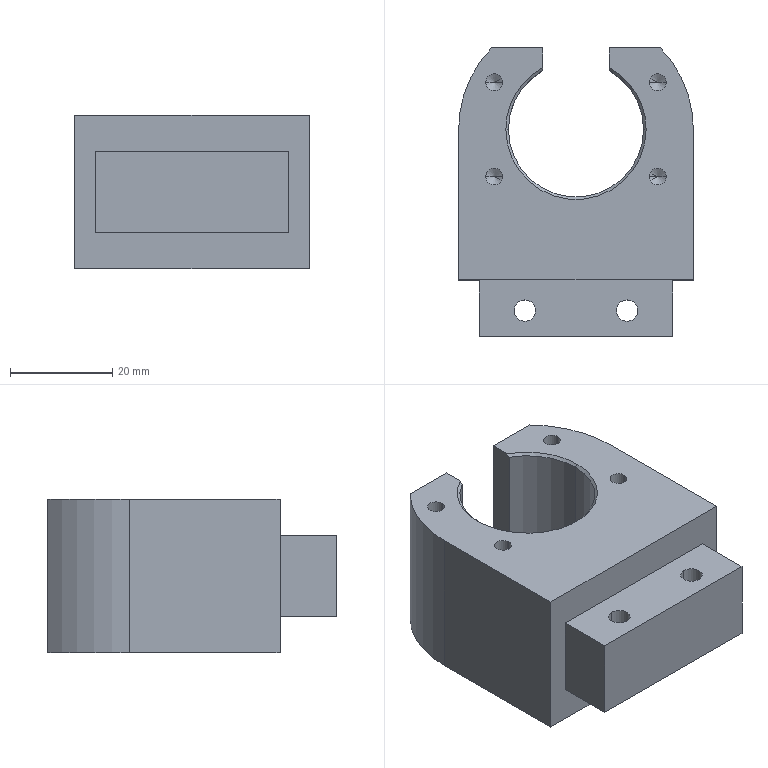Part | NX | features BREP 1 | 1 solid | 45 faces | box 46 x 56.5 x 30 mm | volume 48886 mm3 | cylinder 17 | plane 14 | cone 14 | commonest cylinder face diameters 3.3 x8 4.2 x4 26.5 x3 46 x2
STEP:
#1=CARTESIAN_POINT('',(10.,-37.6,7.));
#2=VERTEX_POINT('',#1);
#3=CARTESIAN_POINT('',(10.,-37.6,23.));
#4=VERTEX_POINT('',#3);
#5=CARTESIAN_POINT('',(10.,-37.6,7.));
#6=DIRECTION('',(0.,0.,-1.));
#7=VECTOR('',#6,1000.);
#8=LINE('',#5,#7);
#9=EDGE_CURVE('',#2,#4,#8,.F.);
#10=ORIENTED_EDGE('',*,*,#9,.T.);
#11=CARTESIAN_POINT('',(10.,-33.4,23.));
#12=VERTEX_POINT('',#11);
#13=CARTESIAN_POINT('',(10.,-35.5,23.));
#14=DIRECTION('',(0.,0.,1.));
#15=DIRECTION('',(1.,0.,0.));
#16=AXIS2_PLACEMENT_3D('',#13,#14,#15);
#17=CIRCLE('',#16,2.1);
#18=EDGE_CURVE('',#4,#12,#17,.T.);
#19=ORIENTED_EDGE('',*,*,#18,.T.);
#20=CARTESIAN_POINT('',(10.,-33.4,7.));
#21=VERTEX_POINT('',#20);
#22=CARTESIAN_POINT('',(10.,-33.4,7.));
#23=DIRECTION('',(0.,0.,-1.));
#24=VECTOR('',#23,1000.);
#25=LINE('',#22,#24);
#26=EDGE_CURVE('',#21,#12,#25,.F.);
#27=ORIENTED_EDGE('',*,*,#26,.F.);
#28=CARTESIAN_POINT('',(10.,-35.5,7.));
#29=DIRECTION('',(0.,0.,-1.));
#30=DIRECTION('',(0.,1.,0.));
#31=AXIS2_PLACEMENT_3D('',#28,#29,#30);
#32=CIRCLE('',#31,2.1);
#33=EDGE_CURVE('',#21,#2,#32,.T.);
#34=ORIENTED_EDGE('',*,*,#33,.T.);
#35=EDGE_LOOP('',(#10,#19,#27,#34));
#36=FACE_BOUND('',#35,.T.);
#37=CARTESIAN_POINT('',(10.,-35.5,7.));
#38=DIRECTION('',(0.,0.,-1.));
#39=DIRECTION('',(0.,1.,0.));
#40=AXIS2_PLACEMENT_3D('',#37,#38,#39);
#41=CYLINDRICAL_SURFACE('',#40,2.1);
#42=ADVANCED_FACE('',(#36),#41,.F.);
#43=CARTESIAN_POINT('',(-10.,-37.6,7.));
#44=VERTEX_POINT('',#43);
#45=CARTESIAN_POINT('',(-10.,-37.6,23.));
#46=VERTEX_POINT('',#45);
#47=CARTESIAN_POINT('',(-10.,-37.6,7.));
#48=DIRECTION('',(0.,0.,-1.));
#49=VECTOR('',#48,1000.);
#50=LINE('',#47,#49);
#51=EDGE_CURVE('',#44,#46,#50,.F.);
#52=ORIENTED_EDGE('',*,*,#51,.T.);
#53=CARTESIAN_POINT('',(-10.,-33.4,23.));
#54=VERTEX_POINT('',#53);
#55=CARTESIAN_POINT('',(-10.,-35.5,23.));
#56=DIRECTION('',(0.,0.,1.));
#57=DIRECTION('',(1.,0.,0.));
#58=AXIS2_PLACEMENT_3D('',#55,#56,#57);
#59=CIRCLE('',#58,2.1);
#60=EDGE_CURVE('',#46,#54,#59,.T.);
#61=ORIENTED_EDGE('',*,*,#60,.T.);
#62=CARTESIAN_POINT('',(-10.,-33.4,7.));
#63=VERTEX_POINT('',#62);
#64=CARTESIAN_POINT('',(-10.,-33.4,7.));
#65=DIRECTION('',(0.,0.,-1.));
#66=VECTOR('',#65,1000.);
#67=LINE('',#64,#66);
#68=EDGE_CURVE('',#63,#54,#67,.F.);
#69=ORIENTED_EDGE('',*,*,#68,.F.);
#70=CARTESIAN_POINT('',(-10.,-35.5,7.));
#71=DIRECTION('',(0.,0.,-1.));
#72=DIRECTION('',(0.,1.,0.));
#73=AXIS2_PLACEMENT_3D('',#70,#71,#72);
#74=CIRCLE('',#73,2.1);
#75=EDGE_CURVE('',#63,#44,#74,.T.);
#76=ORIENTED_EDGE('',*,*,#75,.T.);
#77=EDGE_LOOP('',(#52,#61,#69,#76));
#78=FACE_BOUND('',#77,.T.);
#79=CARTESIAN_POINT('',(-10.,-35.5,7.));
#80=DIRECTION('',(0.,0.,-1.));
#81=DIRECTION('',(0.,1.,0.));
#82=AXIS2_PLACEMENT_3D('',#79,#80,#81);
#83=CYLINDRICAL_SURFACE('',#82,2.1);
#84=ADVANCED_FACE('',(#78),#83,.F.);
#85=CARTESIAN_POINT('',(19.,-40.5,23.));
#86=VERTEX_POINT('',#85);
#87=CARTESIAN_POINT('',(-19.,-40.5,23.));
#88=VERTEX_POINT('',#87);
#89=CARTESIAN_POINT('',(19.,-40.5,23.));
#90=DIRECTION('',(-1.,0.,0.));
#91=VECTOR('',#90,1000.);
#92=LINE('',#89,#91);
#93=EDGE_CURVE('',#86,#88,#92,.T.);
#94=ORIENTED_EDGE('',*,*,#93,.T.);
#95=CARTESIAN_POINT('',(-19.,-40.5,7.));
#96=VERTEX_POINT('',#95);
#97=CARTESIAN_POINT('',(-19.,-40.5,23.));
#98=DIRECTION('',(0.,0.,-1.));
#99=VECTOR('',#98,1000.);
#100=LINE('',#97,#99);
#101=EDGE_CURVE('',#88,#96,#100,.T.);
#102=ORIENTED_EDGE('',*,*,#101,.T.);
#103=CARTESIAN_POINT('',(19.,-40.5,7.));
#104=VERTEX_POINT('',#103);
#105=CARTESIAN_POINT('',(19.,-40.5,7.));
#106=DIRECTION('',(1.,0.,0.));
#107=VECTOR('',#106,1000.);
#108=LINE('',#105,#107);
#109=EDGE_CURVE('',#96,#104,#108,.T.);
#110=ORIENTED_EDGE('',*,*,#109,.T.);
#111=CARTESIAN_POINT('',(19.,-40.5,23.));
#112=DIRECTION('',(0.,0.,1.));
#113=VECTOR('',#112,1000.);
#114=LINE('',#111,#113);
#115=EDGE_CURVE('',#104,#86,#114,.T.);
#116=ORIENTED_EDGE('',*,*,#115,.T.);
#117=EDGE_LOOP('',(#94,#102,#110,#116));
#118=FACE_BOUND('',#117,.T.);
#119=CARTESIAN_POINT('',(23.,-40.5,-61.288));
#120=DIRECTION('',(0.,-1.,0.));
#121=DIRECTION('',(1.,0.,0.));
#122=AXIS2_PLACEMENT_3D('',#119,#120,#121);
#123=PLANE('',#122);
#124=ADVANCED_FACE('',(#118),#123,.T.);
#125=ORIENTED_EDGE('',*,*,#109,.F.);
#126=CARTESIAN_POINT('',(-19.,-29.5,7.));
#127=VERTEX_POINT('',#126);
#128=CARTESIAN_POINT('',(-19.,-29.5,7.));
#129=DIRECTION('',(0.,-1.,0.));
#130=VECTOR('',#129,1000.);
#131=LINE('',#128,#130);
#132=EDGE_CURVE('',#127,#96,#131,.T.);
#133=ORIENTED_EDGE('',*,*,#132,.F.);
#134=CARTESIAN_POINT('',(19.,-29.5,7.));
#135=VERTEX_POINT('',#134);
#136=CARTESIAN_POINT('',(19.,-29.5,7.));
#137=DIRECTION('',(1.,0.,0.));
#138=VECTOR('',#137,1000.);
#139=LINE('',#136,#138);
#140=EDGE_CURVE('',#127,#135,#139,.T.);
#141=ORIENTED_EDGE('',*,*,#140,.T.);
#142=CARTESIAN_POINT('',(19.,-29.5,7.));
#143=DIRECTION('',(0.,-1.,0.));
#144=VECTOR('',#143,1000.);
#145=LINE('',#142,#144);
#146=EDGE_CURVE('',#135,#104,#145,.T.);
#147=ORIENTED_EDGE('',*,*,#146,.T.);
#148=EDGE_LOOP('',(#125,#133,#141,#147));
#149=FACE_BOUND('',#148,.T.);
#150=ORIENTED_EDGE('',*,*,#75,.F.);
#151=CARTESIAN_POINT('',(-10.,-35.5,7.));
#152=DIRECTION('',(0.,0.,-1.));
#153=DIRECTION('',(0.,1.,0.));
#154=AXIS2_PLACEMENT_3D('',#151,#152,#153);
#155=CIRCLE('',#154,2.1);
#156=EDGE_CURVE('',#44,#63,#155,.T.);
#157=ORIENTED_EDGE('',*,*,#156,.F.);
#158=EDGE_LOOP('',(#150,#157));
#159=FACE_BOUND('',#158,.T.);
#160=ORIENTED_EDGE('',*,*,#33,.F.);
#161=CARTESIAN_POINT('',(10.,-35.5,7.));
#162=DIRECTION('',(0.,0.,-1.));
#163=DIRECTION('',(0.,1.,0.));
#164=AXIS2_PLACEMENT_3D('',#161,#162,#163);
#165=CIRCLE('',#164,2.1);
#166=EDGE_CURVE('',#2,#21,#165,.T.);
#167=ORIENTED_EDGE('',*,*,#166,.F.);
#168=EDGE_LOOP('',(#160,#167));
#169=FACE_BOUND('',#168,.T.);
#170=CARTESIAN_POINT('',(19.,-29.5,7.));
#171=DIRECTION('',(0.,0.,-1.));
#172=DIRECTION('',(-1.,0.,0.));
#173=AXIS2_PLACEMENT_3D('',#170,#171,#172);
#174=PLANE('',#173);
#175=ADVANCED_FACE('',(#149,#159,#169),#174,.T.);
#176=ORIENTED_EDGE('',*,*,#115,.F.);
#177=ORIENTED_EDGE('',*,*,#146,.F.);
#178=CARTESIAN_POINT('',(19.,-29.5,23.));
#179=VERTEX_POINT('',#178);
#180=CARTESIAN_POINT('',(19.,-29.5,23.));
#181=DIRECTION('',(0.,0.,1.));
#182=VECTOR('',#181,1000.);
#183=LINE('',#180,#182);
#184=EDGE_CURVE('',#135,#179,#183,.T.);
#185=ORIENTED_EDGE('',*,*,#184,.T.);
#186=CARTESIAN_POINT('',(19.,-29.5,23.));
#187=DIRECTION('',(0.,-1.,0.));
#188=VECTOR('',#187,1000.);
#189=LINE('',#186,#188);
#190=EDGE_CURVE('',#179,#86,#189,.T.);
#191=ORIENTED_EDGE('',*,*,#190,.T.);
#192=EDGE_LOOP('',(#176,#177,#185,#191));
#193=FACE_BOUND('',#192,.T.);
#194=CARTESIAN_POINT('',(19.,-29.5,23.));
#195=DIRECTION('',(1.,0.,0.));
#196=DIRECTION('',(0.,0.,-1.));
#197=AXIS2_PLACEMENT_3D('',#194,#195,#196);
#198=PLANE('',#197);
#199=ADVANCED_FACE('',(#193),#198,.T.);
#200=ORIENTED_EDGE('',*,*,#93,.F.);
#201=ORIENTED_EDGE('',*,*,#190,.F.);
#202=CARTESIAN_POINT('',(-19.,-29.5,23.));
#203=VERTEX_POINT('',#202);
#204=CARTESIAN_POINT('',(19.,-29.5,23.));
#205=DIRECTION('',(-1.,0.,0.));
#206=VECTOR('',#205,1000.);
#207=LINE('',#204,#206);
#208=EDGE_CURVE('',#179,#203,#207,.T.);
#209=ORIENTED_EDGE('',*,*,#208,.T.);
#210=CARTESIAN_POINT('',(-19.,-29.5,23.));
#211=DIRECTION('',(0.,-1.,0.));
#212=VECTOR('',#211,1000.);
#213=LINE('',#210,#212);
#214=EDGE_CURVE('',#203,#88,#213,.T.);
#215=ORIENTED_EDGE('',*,*,#214,.T.);
#216=EDGE_LOOP('',(#200,#201,#209,#215));
#217=FACE_BOUND('',#216,.T.);
#218=CARTESIAN_POINT('',(-10.,-35.5,23.));
#219=DIRECTION('',(0.,0.,1.));
#220=DIRECTION('',(1.,0.,0.));
#221=AXIS2_PLACEMENT_3D('',#218,#219,#220);
#222=CIRCLE('',#221,2.1);
#223=EDGE_CURVE('',#54,#46,#222,.T.);
#224=ORIENTED_EDGE('',*,*,#223,.F.);
#225=ORIENTED_EDGE('',*,*,#60,.F.);
#226=EDGE_LOOP('',(#224,#225));
#227=FACE_BOUND('',#226,.T.);
#228=CARTESIAN_POINT('',(10.,-35.5,23.));
#229=DIRECTION('',(0.,0.,1.));
#230=DIRECTION('',(1.,0.,0.));
#231=AXIS2_PLACEMENT_3D('',#228,#229,#230);
#232=CIRCLE('',#231,2.1);
#233=EDGE_CURVE('',#12,#4,#232,.T.);
#234=ORIENTED_EDGE('',*,*,#233,.F.);
#235=ORIENTED_EDGE('',*,*,#18,.F.);
#236=EDGE_LOOP('',(#234,#235));
#237=FACE_BOUND('',#236,.T.);
#238=CARTESIAN_POINT('',(19.,-29.5,23.));
#239=DIRECTION('',(0.,0.,1.));
#240=DIRECTION('',(1.,0.,0.));
#241=AXIS2_PLACEMENT_3D('',#238,#239,#240);
#242=PLANE('',#241);
#243=ADVANCED_FACE('',(#217,#227,#237),#242,.T.);
#244=ORIENTED_EDGE('',*,*,#101,.F.);
#245=ORIENTED_EDGE('',*,*,#214,.F.);
#246=CARTESIAN_POINT('',(-19.,-29.5,23.));
#247=DIRECTION('',(0.,0.,-1.));
#248=VECTOR('',#247,1000.);
#249=LINE('',#246,#248);
#250=EDGE_CURVE('',#203,#127,#249,.T.);
#251=ORIENTED_EDGE('',*,*,#250,.T.);
#252=ORIENTED_EDGE('',*,*,#132,.T.);
#253=EDGE_LOOP('',(#244,#245,#251,#252));
#254=FACE_BOUND('',#253,.T.);
#255=CARTESIAN_POINT('',(-19.,-29.5,23.));
#256=DIRECTION('',(-1.,0.,0.));
#257=DIRECTION('',(0.,0.,1.));
#258=AXIS2_PLACEMENT_3D('',#255,#256,#257);
#259=PLANE('',#258);
#260=ADVANCED_FACE('',(#254),#259,.T.);
#261=ORIENTED_EDGE('',*,*,#208,.F.);
#262=ORIENTED_EDGE('',*,*,#184,.F.);
#263=ORIENTED_EDGE('',*,*,#140,.F.);
#264=ORIENTED_EDGE('',*,*,#250,.F.);
#265=EDGE_LOOP('',(#261,#262,#263,#264));
#266=FACE_BOUND('',#265,.T.);
#267=CARTESIAN_POINT('',(-23.,-29.5,30.));
#268=VERTEX_POINT('',#267);
#269=CARTESIAN_POINT('',(23.,-29.5,30.));
#270=VERTEX_POINT('',#269);
#271=CARTESIAN_POINT('',(0.,-29.5,30.));
#272=DIRECTION('',(1.,0.,0.));
#273=VECTOR('',#272,1000.);
#274=LINE('',#271,#273);
#275=EDGE_CURVE('',#268,#270,#274,.T.);
#276=ORIENTED_EDGE('',*,*,#275,.F.);
#277=CARTESIAN_POINT('',(-23.,-29.5,0.));
#278=VERTEX_POINT('',#277);
#279=CARTESIAN_POINT('',(-23.,-29.5,-61.288));
#280=DIRECTION('',(0.,0.,1.));
#281=VECTOR('',#280,1000.);
#282=LINE('',#279,#281);
#283=EDGE_CURVE('',#278,#268,#282,.T.);
#284=ORIENTED_EDGE('',*,*,#283,.F.);
#285=CARTESIAN_POINT('',(23.,-29.5,0.));
#286=VERTEX_POINT('',#285);
#287=CARTESIAN_POINT('',(0.,-29.5,0.));
#288=DIRECTION('',(1.,0.,0.));
#289=VECTOR('',#288,1000.);
#290=LINE('',#287,#289);
#291=EDGE_CURVE('',#278,#286,#290,.T.);
#292=ORIENTED_EDGE('',*,*,#291,.T.);
#293=CARTESIAN_POINT('',(23.,-29.5,-61.288));
#294=DIRECTION('',(0.,0.,-1.));
#295=VECTOR('',#294,1000.);
#296=LINE('',#293,#295);
#297=EDGE_CURVE('',#270,#286,#296,.T.);
#298=ORIENTED_EDGE('',*,*,#297,.F.);
#299=EDGE_LOOP('',(#276,#284,#292,#298));
#300=FACE_BOUND('',#299,.T.);
#301=CARTESIAN_POINT('',(0.,-29.5,15.));
#302=DIRECTION('',(0.,-1.,0.));
#303=DIRECTION('',(1.,0.,0.));
#304=AXIS2_PLACEMENT_3D('',#301,#302,#303);
#305=PLANE('',#304);
#306=ADVANCED_FACE('',(#266,#300),#305,.T.);
#307=CARTESIAN_POINT('',(-17.671,-9.25,30.));
#308=VERTEX_POINT('',#307);
#309=CARTESIAN_POINT('',(-17.671,-9.25,19.9));
#310=VERTEX_POINT('',#309);
#311=CARTESIAN_POINT('',(-17.671,-9.25,30.));
#312=DIRECTION('',(0.,0.,1.));
#313=VECTOR('',#312,1000.);
#314=LINE('',#311,#313);
#315=EDGE_CURVE('',#308,#310,#314,.F.);
#316=ORIENTED_EDGE('',*,*,#315,.T.);
#317=CARTESIAN_POINT('',(-14.371,-9.25,19.9));
#318=VERTEX_POINT('',#317);
#319=CARTESIAN_POINT('',(-16.021,-9.25,19.9));
#320=DIRECTION('',(0.,0.,1.));
#321=DIRECTION('',(1.,0.,0.));
#322=AXIS2_PLACEMENT_3D('',#319,#320,#321);
#323=CIRCLE('',#322,1.65);
#324=EDGE_CURVE('',#318,#310,#323,.T.);
#325=ORIENTED_EDGE('',*,*,#324,.F.);
#326=CARTESIAN_POINT('',(-14.371,-9.25,30.));
#327=VERTEX_POINT('',#326);
#328=CARTESIAN_POINT('',(-14.371,-9.25,30.));
#329=DIRECTION('',(0.,0.,1.));
#330=VECTOR('',#329,1000.);
#331=LINE('',#328,#330);
#332=EDGE_CURVE('',#327,#318,#331,.F.);
#333=ORIENTED_EDGE('',*,*,#332,.F.);
#334=CARTESIAN_POINT('',(-16.021,-9.25,30.));
#335=DIRECTION('',(0.,0.,1.));
#336=DIRECTION('',(1.,0.,0.));
#337=AXIS2_PLACEMENT_3D('',#334,#335,#336);
#338=CIRCLE('',#337,1.65);
#339=EDGE_CURVE('',#327,#308,#338,.T.);
#340=ORIENTED_EDGE('',*,*,#339,.T.);
#341=EDGE_LOOP('',(#316,#325,#333,#340));
#342=FACE_BOUND('',#341,.T.);
#343=CARTESIAN_POINT('',(-16.021,-9.25,30.));
#344=DIRECTION('',(0.,0.,1.));
#345=DIRECTION('',(1.,0.,0.));
#346=AXIS2_PLACEMENT_3D('',#343,#344,#345);
#347=CYLINDRICAL_SURFACE('',#346,1.65);
#348=ADVANCED_FACE('',(#342),#347,.F.);
#349=CARTESIAN_POINT('',(-16.021,-9.25,18.909));
#350=VERTEX_POINT('',#349);
#351=CARTESIAN_POINT('',(-17.671,-9.25,19.9));
#352=DIRECTION('',(-0.8572,0.,0.515));
#353=VECTOR('',#352,1000.);
#354=LINE('',#351,#353);
#355=EDGE_CURVE('',#350,#310,#354,.T.);
#356=ORIENTED_EDGE('',*,*,#355,.F.);
#357=CARTESIAN_POINT('',(-14.371,-9.25,19.9));
#358=DIRECTION('',(0.8572,0.,0.515));
#359=VECTOR('',#358,1000.);
#360=LINE('',#357,#359);
#361=EDGE_CURVE('',#350,#318,#360,.T.);
#362=ORIENTED_EDGE('',*,*,#361,.T.);
#363=ORIENTED_EDGE('',*,*,#324,.T.);
#364=EDGE_LOOP('',(#356,#362,#363));
#365=FACE_BOUND('',#364,.T.);
#366=CARTESIAN_POINT('',(-16.021,-9.25,19.9));
#367=DIRECTION('',(0.,0.,1.));
#368=DIRECTION('',(1.,0.,0.));
#369=AXIS2_PLACEMENT_3D('',#366,#367,#368);
#370=CONICAL_SURFACE('',#369,1.65,1.03);
#371=ADVANCED_FACE('',(#365),#370,.F.);
#372=CARTESIAN_POINT('',(14.371,9.25,30.));
#373=VERTEX_POINT('',#372);
#374=CARTESIAN_POINT('',(14.371,9.25,19.9));
#375=VERTEX_POINT('',#374);
#376=CARTESIAN_POINT('',(14.371,9.25,30.));
#377=DIRECTION('',(0.,0.,1.));
#378=VECTOR('',#377,1000.);
#379=LINE('',#376,#378);
#380=EDGE_CURVE('',#373,#375,#379,.F.);
#381=ORIENTED_EDGE('',*,*,#380,.T.);
#382=CARTESIAN_POINT('',(17.671,9.25,19.9));
#383=VERTEX_POINT('',#382);
#384=CARTESIAN_POINT('',(16.021,9.25,19.9));
#385=DIRECTION('',(0.,0.,1.));
#386=DIRECTION('',(1.,0.,0.));
#387=AXIS2_PLACEMENT_3D('',#384,#385,#386);
#388=CIRCLE('',#387,1.65);
#389=EDGE_CURVE('',#383,#375,#388,.T.);
#390=ORIENTED_EDGE('',*,*,#389,.F.);
#391=CARTESIAN_POINT('',(17.671,9.25,30.));
#392=VERTEX_POINT('',#391);
#393=CARTESIAN_POINT('',(17.671,9.25,30.));
#394=DIRECTION('',(0.,0.,1.));
#395=VECTOR('',#394,1000.);
#396=LINE('',#393,#395);
#397=EDGE_CURVE('',#392,#383,#396,.F.);
#398=ORIENTED_EDGE('',*,*,#397,.F.);
#399=CARTESIAN_POINT('',(16.021,9.25,30.));
#400=DIRECTION('',(0.,0.,1.));
#401=DIRECTION('',(1.,0.,0.));
#402=AXIS2_PLACEMENT_3D('',#399,#400,#401);
#403=CIRCLE('',#402,1.65);
#404=EDGE_CURVE('',#392,#373,#403,.T.);
#405=ORIENTED_EDGE('',*,*,#404,.T.);
#406=EDGE_LOOP('',(#381,#390,#398,#405));
#407=FACE_BOUND('',#406,.T.);
#408=CARTESIAN_POINT('',(16.021,9.25,30.));
#409=DIRECTION('',(0.,0.,1.));
#410=DIRECTION('',(1.,0.,0.));
#411=AXIS2_PLACEMENT_3D('',#408,#409,#410);
#412=CYLINDRICAL_SURFACE('',#411,1.65);
#413=ADVANCED_FACE('',(#407),#412,.F.);
#414=CARTESIAN_POINT('',(16.021,9.25,18.909));
#415=VERTEX_POINT('',#414);
#416=CARTESIAN_POINT('',(14.371,9.25,19.9));
#417=DIRECTION('',(-0.8572,0.,0.515));
#418=VECTOR('',#417,1000.);
#419=LINE('',#416,#418);
#420=EDGE_CURVE('',#415,#375,#419,.T.);
#421=ORIENTED_EDGE('',*,*,#420,.F.);
#422=CARTESIAN_POINT('',(17.671,9.25,19.9));
#423=DIRECTION('',(0.8572,0.,0.515));
#424=VECTOR('',#423,1000.);
#425=LINE('',#422,#424);
#426=EDGE_CURVE('',#415,#383,#425,.T.);
#427=ORIENTED_EDGE('',*,*,#426,.T.);
#428=ORIENTED_EDGE('',*,*,#389,.T.);
#429=EDGE_LOOP('',(#421,#427,#428));
#430=FACE_BOUND('',#429,.T.);
#431=CARTESIAN_POINT('',(16.021,9.25,19.9));
#432=DIRECTION('',(0.,0.,1.));
#433=DIRECTION('',(1.,0.,0.));
#434=AXIS2_PLACEMENT_3D('',#431,#432,#433);
#435=CONICAL_SURFACE('',#434,1.65,1.03);
#436=ADVANCED_FACE('',(#430),#435,.F.);
#437=CARTESIAN_POINT('',(14.371,-9.25,30.));
#438=VERTEX_POINT('',#437);
#439=CARTESIAN_POINT('',(14.371,-9.25,19.9));
#440=VERTEX_POINT('',#439);
#441=CARTESIAN_POINT('',(14.371,-9.25,30.));
#442=DIRECTION('',(0.,0.,1.));
#443=VECTOR('',#442,1000.);
#444=LINE('',#441,#443);
#445=EDGE_CURVE('',#438,#440,#444,.F.);
#446=ORIENTED_EDGE('',*,*,#445,.T.);
#447=CARTESIAN_POINT('',(17.671,-9.25,19.9));
#448=VERTEX_POINT('',#447);
#449=CARTESIAN_POINT('',(16.021,-9.25,19.9));
#450=DIRECTION('',(0.,0.,1.));
#451=DIRECTION('',(1.,0.,0.));
#452=AXIS2_PLACEMENT_3D('',#449,#450,#451);
#453=CIRCLE('',#452,1.65);
#454=EDGE_CURVE('',#448,#440,#453,.T.);
#455=ORIENTED_EDGE('',*,*,#454,.F.);
#456=CARTESIAN_POINT('',(17.671,-9.25,30.));
#457=VERTEX_POINT('',#456);
#458=CARTESIAN_POINT('',(17.671,-9.25,30.));
#459=DIRECTION('',(0.,0.,1.));
#460=VECTOR('',#459,1000.);
#461=LINE('',#458,#460);
#462=EDGE_CURVE('',#457,#448,#461,.F.);
#463=ORIENTED_EDGE('',*,*,#462,.F.);
#464=CARTESIAN_POINT('',(16.021,-9.25,30.));
#465=DIRECTION('',(0.,0.,1.));
#466=DIRECTION('',(1.,0.,0.));
#467=AXIS2_PLACEMENT_3D('',#464,#465,#466);
#468=CIRCLE('',#467,1.65);
#469=EDGE_CURVE('',#457,#438,#468,.T.);
#470=ORIENTED_EDGE('',*,*,#469,.T.);
#471=EDGE_LOOP('',(#446,#455,#463,#470));
#472=FACE_BOUND('',#471,.T.);
#473=CARTESIAN_POINT('',(16.021,-9.25,30.));
#474=DIRECTION('',(0.,0.,1.));
#475=DIRECTION('',(1.,0.,0.));
#476=AXIS2_PLACEMENT_3D('',#473,#474,#475);
#477=CYLINDRICAL_SURFACE('',#476,1.65);
#478=ADVANCED_FACE('',(#472),#477,.F.);
#479=CARTESIAN_POINT('',(16.021,-9.25,18.909));
#480=VERTEX_POINT('',#479);
#481=CARTESIAN_POINT('',(14.371,-9.25,19.9));
#482=DIRECTION('',(-0.8572,0.,0.515));
#483=VECTOR('',#482,1000.);
#484=LINE('',#481,#483);
#485=EDGE_CURVE('',#480,#440,#484,.T.);
#486=ORIENTED_EDGE('',*,*,#485,.F.);
#487=CARTESIAN_POINT('',(17.671,-9.25,19.9));
#488=DIRECTION('',(0.8572,0.,0.515));
#489=VECTOR('',#488,1000.);
#490=LINE('',#487,#489);
#491=EDGE_CURVE('',#480,#448,#490,.T.);
#492=ORIENTED_EDGE('',*,*,#491,.T.);
#493=ORIENTED_EDGE('',*,*,#454,.T.);
#494=EDGE_LOOP('',(#486,#492,#493));
#495=FACE_BOUND('',#494,.T.);
#496=CARTESIAN_POINT('',(16.021,-9.25,19.9));
#497=DIRECTION('',(0.,0.,1.));
#498=DIRECTION('',(1.,0.,0.));
#499=AXIS2_PLACEMENT_3D('',#496,#497,#498);
#500=CONICAL_SURFACE('',#499,1.65,1.03);
#501=ADVANCED_FACE('',(#495),#500,.F.);
#502=CARTESIAN_POINT('',(-17.671,9.25,30.));
#503=VERTEX_POINT('',#502);
#504=CARTESIAN_POINT('',(-17.671,9.25,19.9));
#505=VERTEX_POINT('',#504);
#506=CARTESIAN_POINT('',(-17.671,9.25,30.));
#507=DIRECTION('',(0.,0.,1.));
#508=VECTOR('',#507,1000.);
#509=LINE('',#506,#508);
#510=EDGE_CURVE('',#503,#505,#509,.F.);
#511=ORIENTED_EDGE('',*,*,#510,.T.);
#512=CARTESIAN_POINT('',(-14.371,9.25,19.9));
#513=VERTEX_POINT('',#512);
#514=CARTESIAN_POINT('',(-16.021,9.25,19.9));
#515=DIRECTION('',(0.,0.,1.));
#516=DIRECTION('',(1.,0.,0.));
#517=AXIS2_PLACEMENT_3D('',#514,#515,#516);
#518=CIRCLE('',#517,1.65);
#519=EDGE_CURVE('',#513,#505,#518,.T.);
#520=ORIENTED_EDGE('',*,*,#519,.F.);
#521=CARTESIAN_POINT('',(-14.371,9.25,30.));
#522=VERTEX_POINT('',#521);
#523=CARTESIAN_POINT('',(-14.371,9.25,30.));
#524=DIRECTION('',(0.,0.,1.));
#525=VECTOR('',#524,1000.);
#526=LINE('',#523,#525);
#527=EDGE_CURVE('',#522,#513,#526,.F.);
#528=ORIENTED_EDGE('',*,*,#527,.F.);
#529=CARTESIAN_POINT('',(-16.021,9.25,30.));
#530=DIRECTION('',(0.,0.,1.));
#531=DIRECTION('',(1.,0.,0.));
#532=AXIS2_PLACEMENT_3D('',#529,#530,#531);
#533=CIRCLE('',#532,1.65);
#534=EDGE_CURVE('',#522,#503,#533,.T.);
#535=ORIENTED_EDGE('',*,*,#534,.T.);
#536=EDGE_LOOP('',(#511,#520,#528,#535));
#537=FACE_BOUND('',#536,.T.);
#538=CARTESIAN_POINT('',(-16.021,9.25,30.));
#539=DIRECTION('',(0.,0.,1.));
#540=DIRECTION('',(1.,0.,0.));
#541=AXIS2_PLACEMENT_3D('',#538,#539,#540);
#542=CYLINDRICAL_SURFACE('',#541,1.65);
#543=ADVANCED_FACE('',(#537),#542,.F.);
#544=CARTESIAN_POINT('',(-16.021,9.25,18.909));
#545=VERTEX_POINT('',#544);
#546=CARTESIAN_POINT('',(-17.671,9.25,19.9));
#547=DIRECTION('',(-0.8572,0.,0.515));
#548=VECTOR('',#547,1000.);
#549=LINE('',#546,#548);
#550=EDGE_CURVE('',#545,#505,#549,.T.);
#551=ORIENTED_EDGE('',*,*,#550,.F.);
#552=CARTESIAN_POINT('',(-14.371,9.25,19.9));
#553=DIRECTION('',(0.8572,0.,0.515));
#554=VECTOR('',#553,1000.);
#555=LINE('',#552,#554);
#556=EDGE_CURVE('',#545,#513,#555,.T.);
#557=ORIENTED_EDGE('',*,*,#556,.T.);
#558=ORIENTED_EDGE('',*,*,#519,.T.);
#559=EDGE_LOOP('',(#551,#557,#558));
#560=FACE_BOUND('',#559,.T.);
#561=CARTESIAN_POINT('',(-16.021,9.25,19.9));
#562=DIRECTION('',(0.,0.,1.));
#563=DIRECTION('',(1.,0.,0.));
#564=AXIS2_PLACEMENT_3D('',#561,#562,#563);
#565=CONICAL_SURFACE('',#564,1.65,1.03);
#566=ADVANCED_FACE('',(#560),#565,.F.);
#567=CARTESIAN_POINT('',(-13.25,0.,29.5));
#568=VERTEX_POINT('',#567);
#569=CARTESIAN_POINT('',(-13.75,0.,30.));
#570=VERTEX_POINT('',#569);
#571=CARTESIAN_POINT('',(-13.75,0.,30.));
#572=DIRECTION('',(-0.7071,0.,0.7071));
#573=VECTOR('',#572,1000.);
#574=LINE('',#571,#573);
#575=EDGE_CURVE('',#568,#570,#574,.T.);
#576=ORIENTED_EDGE('',*,*,#575,.F.);
#577=CARTESIAN_POINT('',(-6.5,11.546,29.5));
#578=VERTEX_POINT('',#577);
#579=CARTESIAN_POINT('',(0.,0.,29.5));
#580=DIRECTION('',(0.,0.,1.));
#581=DIRECTION('',(1.,0.,0.));
#582=AXIS2_PLACEMENT_3D('',#579,#580,#581);
#583=CIRCLE('',#582,13.25);
#584=EDGE_CURVE('',#578,#568,#583,.T.);
#585=ORIENTED_EDGE('',*,*,#584,.F.);
#586=CARTESIAN_POINT('',(-6.5,12.117,30.));
#587=VERTEX_POINT('',#586);
#588=CARTESIAN_POINT('',(-6.5,12.117,30.));
#589=CARTESIAN_POINT('',(-6.5,11.927,29.833));
#590=CARTESIAN_POINT('',(-6.5,11.737,29.666));
#591=CARTESIAN_POINT('',(-6.5,11.546,29.5));
#592=B_SPLINE_CURVE_WITH_KNOTS('',3,(#588,#589,#590,#591),.UNSPECIFIED.,.F.,.F.,(4,4),(0.,0.0007586),.UNSPECIFIED.);
#593=EDGE_CURVE('',#587,#578,#592,.T.);
#594=ORIENTED_EDGE('',*,*,#593,.F.);
#595=CARTESIAN_POINT('',(0.,0.,30.));
#596=DIRECTION('',(0.,0.,-1.));
#597=DIRECTION('',(1.,0.,0.));
#598=AXIS2_PLACEMENT_3D('',#595,#596,#597);
#599=CIRCLE('',#598,13.75);
#600=EDGE_CURVE('',#570,#587,#599,.T.);
#601=ORIENTED_EDGE('',*,*,#600,.F.);
#602=EDGE_LOOP('',(#576,#585,#594,#601));
#603=FACE_BOUND('',#602,.T.);
#604=CARTESIAN_POINT('',(0.,0.,30.));
#605=DIRECTION('',(0.,0.,1.));
#606=DIRECTION('',(1.,0.,0.));
#607=AXIS2_PLACEMENT_3D('',#604,#605,#606);
#608=CONICAL_SURFACE('',#607,13.75,0.7854);
#609=ADVANCED_FACE('',(#603),#608,.F.);
#610=CARTESIAN_POINT('',(13.25,0.,0.5));
#611=VERTEX_POINT('',#610);
#612=CARTESIAN_POINT('',(13.75,0.,0.));
#613=VERTEX_POINT('',#612);
#614=CARTESIAN_POINT('',(13.25,0.,0.5));
#615=DIRECTION('',(0.7071,0.,-0.7071));
#616=VECTOR('',#615,1000.);
#617=LINE('',#614,#616);
#618=EDGE_CURVE('',#611,#613,#617,.T.);
#619=ORIENTED_EDGE('',*,*,#618,.F.);
#620=CARTESIAN_POINT('',(6.5,11.546,0.5));
#621=VERTEX_POINT('',#620);
#622=CARTESIAN_POINT('',(0.,0.,0.5));
#623=DIRECTION('',(0.,0.,-1.));
#624=DIRECTION('',(1.,0.,0.));
#625=AXIS2_PLACEMENT_3D('',#622,#623,#624);
#626=CIRCLE('',#625,13.25);
#627=EDGE_CURVE('',#621,#611,#626,.T.);
#628=ORIENTED_EDGE('',*,*,#627,.F.);
#629=CARTESIAN_POINT('',(6.5,12.117,0.));
#630=VERTEX_POINT('',#629);
#631=CARTESIAN_POINT('',(6.5,12.117,0.));
#632=CARTESIAN_POINT('',(6.5,11.927,0.1672));
#633=CARTESIAN_POINT('',(6.5,11.737,0.3339));
#634=CARTESIAN_POINT('',(6.5,11.546,0.5));
#635=B_SPLINE_CURVE_WITH_KNOTS('',3,(#631,#632,#633,#634),.UNSPECIFIED.,.F.,.F.,(4,4),(0.,0.0007586),.UNSPECIFIED.);
#636=EDGE_CURVE('',#630,#621,#635,.T.);
#637=ORIENTED_EDGE('',*,*,#636,.F.);
#638=CARTESIAN_POINT('',(0.,0.,0.));
#639=DIRECTION('',(0.,0.,1.));
#640=DIRECTION('',(1.,0.,0.));
#641=AXIS2_PLACEMENT_3D('',#638,#639,#640);
#642=CIRCLE('',#641,13.75);
#643=EDGE_CURVE('',#613,#630,#642,.T.);
#644=ORIENTED_EDGE('',*,*,#643,.F.);
#645=EDGE_LOOP('',(#619,#628,#637,#644));
#646=FACE_BOUND('',#645,.T.);
#647=CARTESIAN_POINT('',(0.,0.,0.5));
#648=DIRECTION('',(0.,0.,-1.));
#649=DIRECTION('',(-1.,0.,0.));
#650=AXIS2_PLACEMENT_3D('',#647,#648,#649);
#651=CONICAL_SURFACE('',#650,13.25,0.7854);
#652=ADVANCED_FACE('',(#646),#651,.F.);
#653=CARTESIAN_POINT('',(-16.523,16.,0.));
#654=VERTEX_POINT('',#653);
#655=CARTESIAN_POINT('',(-6.5,16.,0.));
#656=VERTEX_POINT('',#655);
#657=CARTESIAN_POINT('',(-16.523,16.,0.));
#658=DIRECTION('',(1.,0.,0.));
#659=VECTOR('',#658,1000.);
#660=LINE('',#657,#659);
#661=EDGE_CURVE('',#654,#656,#660,.T.);
#662=ORIENTED_EDGE('',*,*,#661,.F.);
#663=CARTESIAN_POINT('',(-16.523,16.,30.));
#664=VERTEX_POINT('',#663);
#665=CARTESIAN_POINT('',(-16.523,16.,0.));
#666=DIRECTION('',(0.,0.,1.));
#667=VECTOR('',#666,1000.);
#668=LINE('',#665,#667);
#669=EDGE_CURVE('',#654,#664,#668,.T.);
#670=ORIENTED_EDGE('',*,*,#669,.T.);
#671=CARTESIAN_POINT('',(-6.5,16.,30.));
#672=VERTEX_POINT('',#671);
#673=CARTESIAN_POINT('',(-16.523,16.,30.));
#674=DIRECTION('',(1.,0.,0.));
#675=VECTOR('',#674,1000.);
#676=LINE('',#673,#675);
#677=EDGE_CURVE('',#664,#672,#676,.T.);
#678=ORIENTED_EDGE('',*,*,#677,.T.);
#679=CARTESIAN_POINT('',(-6.5,16.,30.));
#680=DIRECTION('',(0.,0.,1.));
#681=VECTOR('',#680,1000.);
#682=LINE('',#679,#681);
#683=EDGE_CURVE('',#656,#672,#682,.T.);
#684=ORIENTED_EDGE('',*,*,#683,.F.);
#685=EDGE_LOOP('',(#662,#670,#678,#684));
#686=FACE_BOUND('',#685,.T.);
#687=CARTESIAN_POINT('',(-16.523,16.,0.));
#688=DIRECTION('',(0.,-1.,0.));
#689=DIRECTION('',(0.,0.,-1.));
#690=AXIS2_PLACEMENT_3D('',#687,#688,#689);
#691=PLANE('',#690);
#692=ADVANCED_FACE('',(#686),#691,.F.);
#693=CARTESIAN_POINT('',(6.5,16.,30.));
#694=VERTEX_POINT('',#693);
#695=CARTESIAN_POINT('',(16.523,16.,30.));
#696=VERTEX_POINT('',#695);
#697=CARTESIAN_POINT('',(-16.523,16.,30.));
#698=DIRECTION('',(1.,0.,0.));
#699=VECTOR('',#698,1000.);
#700=LINE('',#697,#699);
#701=EDGE_CURVE('',#694,#696,#700,.T.);
#702=ORIENTED_EDGE('',*,*,#701,.T.);
#703=CARTESIAN_POINT('',(16.523,16.,0.));
#704=VERTEX_POINT('',#703);
#705=CARTESIAN_POINT('',(16.523,16.,0.));
#706=DIRECTION('',(0.,0.,1.));
#707=VECTOR('',#706,1000.);
#708=LINE('',#705,#707);
#709=EDGE_CURVE('',#704,#696,#708,.T.);
#710=ORIENTED_EDGE('',*,*,#709,.F.);
#711=CARTESIAN_POINT('',(6.5,16.,0.));
#712=VERTEX_POINT('',#711);
#713=CARTESIAN_POINT('',(0.,16.,0.));
#714=DIRECTION('',(1.,0.,0.));
#715=VECTOR('',#714,1000.);
#716=LINE('',#713,#715);
#717=EDGE_CURVE('',#712,#704,#716,.T.);
#718=ORIENTED_EDGE('',*,*,#717,.F.);
#719=CARTESIAN_POINT('',(6.5,16.,30.));
#720=DIRECTION('',(0.,0.,-1.));
#721=VECTOR('',#720,1000.);
#722=LINE('',#719,#721);
#723=EDGE_CURVE('',#694,#712,#722,.T.);
#724=ORIENTED_EDGE('',*,*,#723,.F.);
#725=EDGE_LOOP('',(#702,#710,#718,#724));
#726=FACE_BOUND('',#725,.T.);
#727=CARTESIAN_POINT('',(-16.523,16.,0.));
#728=DIRECTION('',(0.,-1.,0.));
#729=DIRECTION('',(0.,0.,-1.));
#730=AXIS2_PLACEMENT_3D('',#727,#728,#729);
#731=PLANE('',#730);
#732=ADVANCED_FACE('',(#726),#731,.F.);
#733=CARTESIAN_POINT('',(-6.5,11.546,0.5));
#734=VERTEX_POINT('',#733);
#735=CARTESIAN_POINT('',(-6.5,11.546,30.));
#736=DIRECTION('',(0.,0.,-1.));
#737=VECTOR('',#736,1000.);
#738=LINE('',#735,#737);
#739=EDGE_CURVE('',#578,#734,#738,.T.);
#740=ORIENTED_EDGE('',*,*,#739,.T.);
#741=CARTESIAN_POINT('',(-6.5,12.117,0.));
#742=VERTEX_POINT('',#741);
#743=CARTESIAN_POINT('',(-6.5,11.546,0.5));
#744=CARTESIAN_POINT('',(-6.5,11.737,0.3339));
#745=CARTESIAN_POINT('',(-6.5,11.927,0.1672));
#746=CARTESIAN_POINT('',(-6.5,12.117,0.));
#747=B_SPLINE_CURVE_WITH_KNOTS('',3,(#743,#744,#745,#746),.UNSPECIFIED.,.F.,.F.,(4,4),(0.,0.0007586),.UNSPECIFIED.);
#748=EDGE_CURVE('',#734,#742,#747,.T.);
#749=ORIENTED_EDGE('',*,*,#748,.T.);
#750=CARTESIAN_POINT('',(-6.5,22.062,0.));
#751=DIRECTION('',(0.,1.,0.));
#752=VECTOR('',#751,1000.);
#753=LINE('',#750,#752);
#754=EDGE_CURVE('',#742,#656,#753,.T.);
#755=ORIENTED_EDGE('',*,*,#754,.T.);
#756=ORIENTED_EDGE('',*,*,#683,.T.);
#757=CARTESIAN_POINT('',(-6.5,22.062,30.));
#758=DIRECTION('',(0.,1.,0.));
#759=VECTOR('',#758,1000.);
#760=LINE('',#757,#759);
#761=EDGE_CURVE('',#587,#672,#760,.T.);
#762=ORIENTED_EDGE('',*,*,#761,.F.);
#763=ORIENTED_EDGE('',*,*,#593,.T.);
#764=EDGE_LOOP('',(#740,#749,#755,#756,#762,#763));
#765=FACE_BOUND('',#764,.T.);
#766=CARTESIAN_POINT('',(-6.5,22.062,30.));
#767=DIRECTION('',(-1.,0.,0.));
#768=DIRECTION('',(0.,-1.,0.));
#769=AXIS2_PLACEMENT_3D('',#766,#767,#768);
#770=PLANE('',#769);
#771=ADVANCED_FACE('',(#765),#770,.F.);
#772=CARTESIAN_POINT('',(13.25,0.,29.5));
#773=VERTEX_POINT('',#772);
#774=CARTESIAN_POINT('',(13.25,0.,30.));
#775=DIRECTION('',(0.,0.,-1.));
#776=VECTOR('',#775,1000.);
#777=LINE('',#774,#776);
#778=EDGE_CURVE('',#773,#611,#777,.T.);
#779=ORIENTED_EDGE('',*,*,#778,.F.);
#780=CARTESIAN_POINT('',(6.5,11.546,29.5));
#781=VERTEX_POINT('',#780);
#782=CARTESIAN_POINT('',(0.,0.,29.5));
#783=DIRECTION('',(0.,0.,1.));
#784=DIRECTION('',(1.,0.,0.));
#785=AXIS2_PLACEMENT_3D('',#782,#783,#784);
#786=CIRCLE('',#785,13.25);
#787=EDGE_CURVE('',#773,#781,#786,.T.);
#788=ORIENTED_EDGE('',*,*,#787,.T.);
#789=CARTESIAN_POINT('',(6.5,11.546,30.));
#790=DIRECTION('',(0.,0.,-1.));
#791=VECTOR('',#790,1000.);
#792=LINE('',#789,#791);
#793=EDGE_CURVE('',#781,#621,#792,.T.);
#794=ORIENTED_EDGE('',*,*,#793,.T.);
#795=ORIENTED_EDGE('',*,*,#627,.T.);
#796=EDGE_LOOP('',(#779,#788,#794,#795));
#797=FACE_BOUND('',#796,.T.);
#798=CARTESIAN_POINT('',(0.,0.,30.));
#799=DIRECTION('',(0.,0.,-1.));
#800=DIRECTION('',(-1.,0.,0.));
#801=AXIS2_PLACEMENT_3D('',#798,#799,#800);
#802=CYLINDRICAL_SURFACE('',#801,13.25);
#803=ADVANCED_FACE('',(#797),#802,.F.);
#804=CARTESIAN_POINT('',(6.5,22.062,0.));
#805=DIRECTION('',(0.,-1.,0.));
#806=VECTOR('',#805,1000.);
#807=LINE('',#804,#806);
#808=EDGE_CURVE('',#712,#630,#807,.T.);
#809=ORIENTED_EDGE('',*,*,#808,.T.);
#810=ORIENTED_EDGE('',*,*,#636,.T.);
#811=ORIENTED_EDGE('',*,*,#793,.F.);
#812=CARTESIAN_POINT('',(6.5,12.117,30.));
#813=VERTEX_POINT('',#812);
#814=CARTESIAN_POINT('',(6.5,11.546,29.5));
#815=CARTESIAN_POINT('',(6.5,11.737,29.666));
#816=CARTESIAN_POINT('',(6.5,11.927,29.833));
#817=CARTESIAN_POINT('',(6.5,12.117,30.));
#818=B_SPLINE_CURVE_WITH_KNOTS('',3,(#814,#815,#816,#817),.UNSPECIFIED.,.F.,.F.,(4,4),(0.,0.0007586),.UNSPECIFIED.);
#819=EDGE_CURVE('',#781,#813,#818,.T.);
#820=ORIENTED_EDGE('',*,*,#819,.T.);
#821=CARTESIAN_POINT('',(6.5,22.062,30.));
#822=DIRECTION('',(0.,-1.,0.));
#823=VECTOR('',#822,1000.);
#824=LINE('',#821,#823);
#825=EDGE_CURVE('',#694,#813,#824,.T.);
#826=ORIENTED_EDGE('',*,*,#825,.F.);
#827=ORIENTED_EDGE('',*,*,#723,.T.);
#828=EDGE_LOOP('',(#809,#810,#811,#820,#826,#827));
#829=FACE_BOUND('',#828,.T.);
#830=CARTESIAN_POINT('',(6.5,22.062,30.));
#831=DIRECTION('',(1.,0.,0.));
#832=DIRECTION('',(0.,1.,0.));
#833=AXIS2_PLACEMENT_3D('',#830,#831,#832);
#834=PLANE('',#833);
#835=ADVANCED_FACE('',(#829),#834,.F.);
#836=CARTESIAN_POINT('',(23.,0.,0.));
#837=VERTEX_POINT('',#836);
#838=CARTESIAN_POINT('',(0.,0.,0.));
#839=DIRECTION('',(0.,0.,1.));
#840=DIRECTION('',(1.,0.,0.));
#841=AXIS2_PLACEMENT_3D('',#838,#839,#840);
#842=CIRCLE('',#841,23.);
#843=EDGE_CURVE('',#837,#704,#842,.T.);
#844=ORIENTED_EDGE('',*,*,#843,.T.);
#845=ORIENTED_EDGE('',*,*,#709,.T.);
#846=CARTESIAN_POINT('',(23.,0.,30.));
#847=VERTEX_POINT('',#846);
#848=CARTESIAN_POINT('',(0.,0.,30.));
#849=DIRECTION('',(0.,0.,1.));
#850=DIRECTION('',(1.,0.,0.));
#851=AXIS2_PLACEMENT_3D('',#848,#849,#850);
#852=CIRCLE('',#851,23.);
#853=EDGE_CURVE('',#847,#696,#852,.T.);
#854=ORIENTED_EDGE('',*,*,#853,.F.);
#855=CARTESIAN_POINT('',(23.,0.,-61.288));
#856=DIRECTION('',(0.,0.,1.));
#857=VECTOR('',#856,1000.);
#858=LINE('',#855,#857);
#859=EDGE_CURVE('',#837,#847,#858,.T.);
#860=ORIENTED_EDGE('',*,*,#859,.F.);
#861=EDGE_LOOP('',(#844,#845,#854,#860));
#862=FACE_BOUND('',#861,.T.);
#863=CARTESIAN_POINT('',(0.,0.,30.));
#864=DIRECTION('',(0.,0.,-1.));
#865=DIRECTION('',(-1.,0.,0.));
#866=AXIS2_PLACEMENT_3D('',#863,#864,#865);
#867=CYLINDRICAL_SURFACE('',#866,23.);
#868=ADVANCED_FACE('',(#862),#867,.T.);
#869=CARTESIAN_POINT('',(-23.,0.,30.));
#870=VERTEX_POINT('',#869);
#871=CARTESIAN_POINT('',(0.,0.,30.));
#872=DIRECTION('',(0.,0.,1.));
#873=DIRECTION('',(1.,0.,0.));
#874=AXIS2_PLACEMENT_3D('',#871,#872,#873);
#875=CIRCLE('',#874,23.);
#876=EDGE_CURVE('',#664,#870,#875,.T.);
#877=ORIENTED_EDGE('',*,*,#876,.F.);
#878=ORIENTED_EDGE('',*,*,#669,.F.);
#879=CARTESIAN_POINT('',(-23.,0.,0.));
#880=VERTEX_POINT('',#879);
#881=CARTESIAN_POINT('',(0.,0.,0.));
#882=DIRECTION('',(0.,0.,1.));
#883=DIRECTION('',(1.,0.,0.));
#884=AXIS2_PLACEMENT_3D('',#881,#882,#883);
#885=CIRCLE('',#884,23.);
#886=EDGE_CURVE('',#654,#880,#885,.T.);
#887=ORIENTED_EDGE('',*,*,#886,.T.);
#888=CARTESIAN_POINT('',(-23.,0.,-61.288));
#889=DIRECTION('',(0.,0.,1.));
#890=VECTOR('',#889,1000.);
#891=LINE('',#888,#890);
#892=EDGE_CURVE('',#880,#870,#891,.T.);
#893=ORIENTED_EDGE('',*,*,#892,.T.);
#894=EDGE_LOOP('',(#877,#878,#887,#893));
#895=FACE_BOUND('',#894,.T.);
#896=CARTESIAN_POINT('',(0.,0.,30.));
#897=DIRECTION('',(0.,0.,-1.));
#898=DIRECTION('',(-1.,0.,0.));
#899=AXIS2_PLACEMENT_3D('',#896,#897,#898);
#900=CYLINDRICAL_SURFACE('',#899,23.);
#901=ADVANCED_FACE('',(#895),#900,.T.);
#902=CARTESIAN_POINT('',(-23.,0.,0.));
#903=DIRECTION('',(0.,1.,0.));
#904=VECTOR('',#903,1000.);
#905=LINE('',#902,#904);
#906=EDGE_CURVE('',#278,#880,#905,.T.);
#907=ORIENTED_EDGE('',*,*,#906,.F.);
#908=ORIENTED_EDGE('',*,*,#283,.T.);
#909=CARTESIAN_POINT('',(-23.,0.,30.));
#910=DIRECTION('',(0.,-1.,0.));
#911=VECTOR('',#910,1000.);
#912=LINE('',#909,#911);
#913=EDGE_CURVE('',#870,#268,#912,.T.);
#914=ORIENTED_EDGE('',*,*,#913,.F.);
#915=ORIENTED_EDGE('',*,*,#892,.F.);
#916=EDGE_LOOP('',(#907,#908,#914,#915));
#917=FACE_BOUND('',#916,.T.);
#918=CARTESIAN_POINT('',(-23.,0.,-61.288));
#919=DIRECTION('',(-1.,0.,0.));
#920=DIRECTION('',(0.,-1.,0.));
#921=AXIS2_PLACEMENT_3D('',#918,#919,#920);
#922=PLANE('',#921);
#923=ADVANCED_FACE('',(#917),#922,.T.);
#924=CARTESIAN_POINT('',(23.,0.,30.));
#925=DIRECTION('',(0.,1.,0.));
#926=VECTOR('',#925,1000.);
#927=LINE('',#924,#926);
#928=EDGE_CURVE('',#270,#847,#927,.T.);
#929=ORIENTED_EDGE('',*,*,#928,.F.);
#930=ORIENTED_EDGE('',*,*,#297,.T.);
#931=CARTESIAN_POINT('',(23.,0.,0.));
#932=DIRECTION('',(0.,-1.,0.));
#933=VECTOR('',#932,1000.);
#934=LINE('',#931,#933);
#935=EDGE_CURVE('',#837,#286,#934,.T.);
#936=ORIENTED_EDGE('',*,*,#935,.F.);
#937=ORIENTED_EDGE('',*,*,#859,.T.);
#938=EDGE_LOOP('',(#929,#930,#936,#937));
#939=FACE_BOUND('',#938,.T.);
#940=CARTESIAN_POINT('',(23.,0.,-61.288));
#941=DIRECTION('',(1.,0.,0.));
#942=DIRECTION('',(0.,1.,0.));
#943=AXIS2_PLACEMENT_3D('',#940,#941,#942);
#944=PLANE('',#943);
#945=ADVANCED_FACE('',(#939),#944,.T.);
#946=ORIENTED_EDGE('',*,*,#291,.F.);
#947=ORIENTED_EDGE('',*,*,#906,.T.);
#948=ORIENTED_EDGE('',*,*,#886,.F.);
#949=ORIENTED_EDGE('',*,*,#661,.T.);
#950=ORIENTED_EDGE('',*,*,#754,.F.);
#951=CARTESIAN_POINT('',(-13.75,0.,0.));
#952=VERTEX_POINT('',#951);
#953=CARTESIAN_POINT('',(0.,0.,0.));
#954=DIRECTION('',(0.,0.,1.));
#955=DIRECTION('',(1.,0.,0.));
#956=AXIS2_PLACEMENT_3D('',#953,#954,#955);
#957=CIRCLE('',#956,13.75);
#958=EDGE_CURVE('',#742,#952,#957,.T.);
#959=ORIENTED_EDGE('',*,*,#958,.T.);
#960=CARTESIAN_POINT('',(0.,0.,0.));
#961=DIRECTION('',(0.,0.,1.));
#962=DIRECTION('',(1.,0.,0.));
#963=AXIS2_PLACEMENT_3D('',#960,#961,#962);
#964=CIRCLE('',#963,13.75);
#965=EDGE_CURVE('',#952,#613,#964,.T.);
#966=ORIENTED_EDGE('',*,*,#965,.T.);
#967=ORIENTED_EDGE('',*,*,#643,.T.);
#968=ORIENTED_EDGE('',*,*,#808,.F.);
#969=ORIENTED_EDGE('',*,*,#717,.T.);
#970=ORIENTED_EDGE('',*,*,#843,.F.);
#971=ORIENTED_EDGE('',*,*,#935,.T.);
#972=EDGE_LOOP('',(#946,#947,#948,#949,#950,#959,#966,#967,#968,#969,#970,#971));
#973=FACE_BOUND('',#972,.T.);
#974=CARTESIAN_POINT('',(0.,0.,0.));
#975=DIRECTION('',(0.,0.,1.));
#976=DIRECTION('',(1.,0.,0.));
#977=AXIS2_PLACEMENT_3D('',#974,#975,#976);
#978=PLANE('',#977);
#979=ADVANCED_FACE('',(#973),#978,.F.);
#980=ORIENTED_EDGE('',*,*,#913,.T.);
#981=ORIENTED_EDGE('',*,*,#275,.T.);
#982=ORIENTED_EDGE('',*,*,#928,.T.);
#983=ORIENTED_EDGE('',*,*,#853,.T.);
#984=ORIENTED_EDGE('',*,*,#701,.F.);
#985=ORIENTED_EDGE('',*,*,#825,.T.);
#986=CARTESIAN_POINT('',(13.75,0.,30.));
#987=VERTEX_POINT('',#986);
#988=CARTESIAN_POINT('',(0.,0.,30.));
#989=DIRECTION('',(0.,0.,-1.));
#990=DIRECTION('',(1.,0.,0.));
#991=AXIS2_PLACEMENT_3D('',#988,#989,#990);
#992=CIRCLE('',#991,13.75);
#993=EDGE_CURVE('',#813,#987,#992,.T.);
#994=ORIENTED_EDGE('',*,*,#993,.T.);
#995=CARTESIAN_POINT('',(0.,0.,30.));
#996=DIRECTION('',(0.,0.,-1.));
#997=DIRECTION('',(1.,0.,0.));
#998=AXIS2_PLACEMENT_3D('',#995,#996,#997);
#999=CIRCLE('',#998,13.75);
#1000=EDGE_CURVE('',#987,#570,#999,.T.);
#1001=ORIENTED_EDGE('',*,*,#1000,.T.);
#1002=ORIENTED_EDGE('',*,*,#600,.T.);
#1003=ORIENTED_EDGE('',*,*,#761,.T.);
#1004=ORIENTED_EDGE('',*,*,#677,.F.);
#1005=ORIENTED_EDGE('',*,*,#876,.T.);
#1006=EDGE_LOOP('',(#980,#981,#982,#983,#984,#985,#994,#1001,#1002,#1003,#1004,#1005));
#1007=FACE_BOUND('',#1006,.T.);
#1008=ORIENTED_EDGE('',*,*,#534,.F.);
#1009=CARTESIAN_POINT('',(-16.021,9.25,30.));
#1010=DIRECTION('',(0.,0.,1.));
#1011=DIRECTION('',(1.,0.,0.));
#1012=AXIS2_PLACEMENT_3D('',#1009,#1010,#1011);
#1013=CIRCLE('',#1012,1.65);
#1014=EDGE_CURVE('',#503,#522,#1013,.T.);
#1015=ORIENTED_EDGE('',*,*,#1014,.F.);
#1016=EDGE_LOOP('',(#1008,#1015));
#1017=FACE_BOUND('',#1016,.T.);
#1018=ORIENTED_EDGE('',*,*,#469,.F.);
#1019=CARTESIAN_POINT('',(16.021,-9.25,30.));
#1020=DIRECTION('',(0.,0.,1.));
#1021=DIRECTION('',(1.,0.,0.));
#1022=AXIS2_PLACEMENT_3D('',#1019,#1020,#1021);
#1023=CIRCLE('',#1022,1.65);
#1024=EDGE_CURVE('',#438,#457,#1023,.T.);
#1025=ORIENTED_EDGE('',*,*,#1024,.F.);
#1026=EDGE_LOOP('',(#1018,#1025));
#1027=FACE_BOUND('',#1026,.T.);
#1028=ORIENTED_EDGE('',*,*,#404,.F.);
#1029=CARTESIAN_POINT('',(16.021,9.25,30.));
#1030=DIRECTION('',(0.,0.,1.));
#1031=DIRECTION('',(1.,0.,0.));
#1032=AXIS2_PLACEMENT_3D('',#1029,#1030,#1031);
#1033=CIRCLE('',#1032,1.65);
#1034=EDGE_CURVE('',#373,#392,#1033,.T.);
#1035=ORIENTED_EDGE('',*,*,#1034,.F.);
#1036=EDGE_LOOP('',(#1028,#1035));
#1037=FACE_BOUND('',#1036,.T.);
#1038=ORIENTED_EDGE('',*,*,#339,.F.);
#1039=CARTESIAN_POINT('',(-16.021,-9.25,30.));
#1040=DIRECTION('',(0.,0.,1.));
#1041=DIRECTION('',(1.,0.,0.));
#1042=AXIS2_PLACEMENT_3D('',#1039,#1040,#1041);
#1043=CIRCLE('',#1042,1.65);
#1044=EDGE_CURVE('',#308,#327,#1043,.T.);
#1045=ORIENTED_EDGE('',*,*,#1044,.F.);
#1046=EDGE_LOOP('',(#1038,#1045));
#1047=FACE_BOUND('',#1046,.T.);
#1048=CARTESIAN_POINT('',(0.,0.,30.));
#1049=DIRECTION('',(0.,0.,1.));
#1050=DIRECTION('',(1.,0.,0.));
#1051=AXIS2_PLACEMENT_3D('',#1048,#1049,#1050);
#1052=PLANE('',#1051);
#1053=ADVANCED_FACE('',(#1007,#1017,#1027,#1037,#1047),#1052,.T.);
#1054=ORIENTED_EDGE('',*,*,#584,.T.);
#1055=CARTESIAN_POINT('',(-13.25,0.,0.5));
#1056=VERTEX_POINT('',#1055);
#1057=CARTESIAN_POINT('',(-13.25,0.,30.));
#1058=DIRECTION('',(0.,0.,-1.));
#1059=VECTOR('',#1058,1000.);
#1060=LINE('',#1057,#1059);
#1061=EDGE_CURVE('',#568,#1056,#1060,.T.);
#1062=ORIENTED_EDGE('',*,*,#1061,.T.);
#1063=CARTESIAN_POINT('',(0.,0.,0.5));
#1064=DIRECTION('',(0.,0.,-1.));
#1065=DIRECTION('',(1.,0.,0.));
#1066=AXIS2_PLACEMENT_3D('',#1063,#1064,#1065);
#1067=CIRCLE('',#1066,13.25);
#1068=EDGE_CURVE('',#1056,#734,#1067,.T.);
#1069=ORIENTED_EDGE('',*,*,#1068,.T.);
#1070=ORIENTED_EDGE('',*,*,#739,.F.);
#1071=EDGE_LOOP('',(#1054,#1062,#1069,#1070));
#1072=FACE_BOUND('',#1071,.T.);
#1073=CARTESIAN_POINT('',(0.,0.,30.));
#1074=DIRECTION('',(0.,0.,-1.));
#1075=DIRECTION('',(-1.,0.,0.));
#1076=AXIS2_PLACEMENT_3D('',#1073,#1074,#1075);
#1077=CYLINDRICAL_SURFACE('',#1076,13.25);
#1078=ADVANCED_FACE('',(#1072),#1077,.F.);
#1079=CARTESIAN_POINT('',(0.,0.,29.5));
#1080=DIRECTION('',(0.,0.,1.));
#1081=DIRECTION('',(1.,0.,0.));
#1082=AXIS2_PLACEMENT_3D('',#1079,#1080,#1081);
#1083=CIRCLE('',#1082,13.25);
#1084=EDGE_CURVE('',#568,#773,#1083,.T.);
#1085=ORIENTED_EDGE('',*,*,#1084,.T.);
#1086=ORIENTED_EDGE('',*,*,#778,.T.);
#1087=CARTESIAN_POINT('',(0.,0.,0.5));
#1088=DIRECTION('',(0.,0.,-1.));
#1089=DIRECTION('',(1.,0.,0.));
#1090=AXIS2_PLACEMENT_3D('',#1087,#1088,#1089);
#1091=CIRCLE('',#1090,13.25);
#1092=EDGE_CURVE('',#611,#1056,#1091,.T.);
#1093=ORIENTED_EDGE('',*,*,#1092,.T.);
#1094=ORIENTED_EDGE('',*,*,#1061,.F.);
#1095=EDGE_LOOP('',(#1085,#1086,#1093,#1094));
#1096=FACE_BOUND('',#1095,.T.);
#1097=CARTESIAN_POINT('',(0.,0.,30.));
#1098=DIRECTION('',(0.,0.,-1.));
#1099=DIRECTION('',(-1.,0.,0.));
#1100=AXIS2_PLACEMENT_3D('',#1097,#1098,#1099);
#1101=CYLINDRICAL_SURFACE('',#1100,13.25);
#1102=ADVANCED_FACE('',(#1096),#1101,.F.);
#1103=ORIENTED_EDGE('',*,*,#1068,.F.);
#1104=CARTESIAN_POINT('',(-13.25,0.,0.5));
#1105=DIRECTION('',(-0.7071,0.,-0.7071));
#1106=VECTOR('',#1105,1000.);
#1107=LINE('',#1104,#1106);
#1108=EDGE_CURVE('',#1056,#952,#1107,.T.);
#1109=ORIENTED_EDGE('',*,*,#1108,.T.);
#1110=ORIENTED_EDGE('',*,*,#958,.F.);
#1111=ORIENTED_EDGE('',*,*,#748,.F.);
#1112=EDGE_LOOP('',(#1103,#1109,#1110,#1111));
#1113=FACE_BOUND('',#1112,.T.);
#1114=CARTESIAN_POINT('',(0.,0.,0.5));
#1115=DIRECTION('',(0.,0.,-1.));
#1116=DIRECTION('',(-1.,0.,0.));
#1117=AXIS2_PLACEMENT_3D('',#1114,#1115,#1116);
#1118=CONICAL_SURFACE('',#1117,13.25,0.7854);
#1119=ADVANCED_FACE('',(#1113),#1118,.F.);
#1120=ORIENTED_EDGE('',*,*,#1092,.F.);
#1121=ORIENTED_EDGE('',*,*,#618,.T.);
#1122=ORIENTED_EDGE('',*,*,#965,.F.);
#1123=ORIENTED_EDGE('',*,*,#1108,.F.);
#1124=EDGE_LOOP('',(#1120,#1121,#1122,#1123));
#1125=FACE_BOUND('',#1124,.T.);
#1126=CARTESIAN_POINT('',(0.,0.,0.5));
#1127=DIRECTION('',(0.,0.,-1.));
#1128=DIRECTION('',(-1.,0.,0.));
#1129=AXIS2_PLACEMENT_3D('',#1126,#1127,#1128);
#1130=CONICAL_SURFACE('',#1129,13.25,0.7854);
#1131=ADVANCED_FACE('',(#1125),#1130,.F.);
#1132=ORIENTED_EDGE('',*,*,#787,.F.);
#1133=CARTESIAN_POINT('',(13.75,0.,30.));
#1134=DIRECTION('',(0.7071,0.,0.7071));
#1135=VECTOR('',#1134,1000.);
#1136=LINE('',#1133,#1135);
#1137=EDGE_CURVE('',#773,#987,#1136,.T.);
#1138=ORIENTED_EDGE('',*,*,#1137,.T.);
#1139=ORIENTED_EDGE('',*,*,#993,.F.);
#1140=ORIENTED_EDGE('',*,*,#819,.F.);
#1141=EDGE_LOOP('',(#1132,#1138,#1139,#1140));
#1142=FACE_BOUND('',#1141,.T.);
#1143=CARTESIAN_POINT('',(0.,0.,30.));
#1144=DIRECTION('',(0.,0.,1.));
#1145=DIRECTION('',(1.,0.,0.));
#1146=AXIS2_PLACEMENT_3D('',#1143,#1144,#1145);
#1147=CONICAL_SURFACE('',#1146,13.75,0.7854);
#1148=ADVANCED_FACE('',(#1142),#1147,.F.);
#1149=ORIENTED_EDGE('',*,*,#1084,.F.);
#1150=ORIENTED_EDGE('',*,*,#575,.T.);
#1151=ORIENTED_EDGE('',*,*,#1000,.F.);
#1152=ORIENTED_EDGE('',*,*,#1137,.F.);
#1153=EDGE_LOOP('',(#1149,#1150,#1151,#1152));
#1154=FACE_BOUND('',#1153,.T.);
#1155=CARTESIAN_POINT('',(0.,0.,30.));
#1156=DIRECTION('',(0.,0.,1.));
#1157=DIRECTION('',(1.,0.,0.));
#1158=AXIS2_PLACEMENT_3D('',#1155,#1156,#1157);
#1159=CONICAL_SURFACE('',#1158,13.75,0.7854);
#1160=ADVANCED_FACE('',(#1154),#1159,.F.);
#1161=ORIENTED_EDGE('',*,*,#556,.F.);
#1162=ORIENTED_EDGE('',*,*,#550,.T.);
#1163=CARTESIAN_POINT('',(-16.021,9.25,19.9));
#1164=DIRECTION('',(0.,0.,1.));
#1165=DIRECTION('',(1.,0.,0.));
#1166=AXIS2_PLACEMENT_3D('',#1163,#1164,#1165);
#1167=CIRCLE('',#1166,1.65);
#1168=EDGE_CURVE('',#505,#513,#1167,.T.);
#1169=ORIENTED_EDGE('',*,*,#1168,.T.);
#1170=EDGE_LOOP('',(#1161,#1162,#1169));
#1171=FACE_BOUND('',#1170,.T.);
#1172=CARTESIAN_POINT('',(-16.021,9.25,19.9));
#1173=DIRECTION('',(0.,0.,1.));
#1174=DIRECTION('',(1.,0.,0.));
#1175=AXIS2_PLACEMENT_3D('',#1172,#1173,#1174);
#1176=CONICAL_SURFACE('',#1175,1.65,1.03);
#1177=ADVANCED_FACE('',(#1171),#1176,.F.);
#1178=ORIENTED_EDGE('',*,*,#1168,.F.);
#1179=ORIENTED_EDGE('',*,*,#510,.F.);
#1180=ORIENTED_EDGE('',*,*,#1014,.T.);
#1181=ORIENTED_EDGE('',*,*,#527,.T.);
#1182=EDGE_LOOP('',(#1178,#1179,#1180,#1181));
#1183=FACE_BOUND('',#1182,.T.);
#1184=CARTESIAN_POINT('',(-16.021,9.25,30.));
#1185=DIRECTION('',(0.,0.,1.));
#1186=DIRECTION('',(1.,0.,0.));
#1187=AXIS2_PLACEMENT_3D('',#1184,#1185,#1186);
#1188=CYLINDRICAL_SURFACE('',#1187,1.65);
#1189=ADVANCED_FACE('',(#1183),#1188,.F.);
#1190=ORIENTED_EDGE('',*,*,#491,.F.);
#1191=ORIENTED_EDGE('',*,*,#485,.T.);
#1192=CARTESIAN_POINT('',(16.021,-9.25,19.9));
#1193=DIRECTION('',(0.,0.,1.));
#1194=DIRECTION('',(1.,0.,0.));
#1195=AXIS2_PLACEMENT_3D('',#1192,#1193,#1194);
#1196=CIRCLE('',#1195,1.65);
#1197=EDGE_CURVE('',#440,#448,#1196,.T.);
#1198=ORIENTED_EDGE('',*,*,#1197,.T.);
#1199=EDGE_LOOP('',(#1190,#1191,#1198));
#1200=FACE_BOUND('',#1199,.T.);
#1201=CARTESIAN_POINT('',(16.021,-9.25,19.9));
#1202=DIRECTION('',(0.,0.,1.));
#1203=DIRECTION('',(1.,0.,0.));
#1204=AXIS2_PLACEMENT_3D('',#1201,#1202,#1203);
#1205=CONICAL_SURFACE('',#1204,1.65,1.03);
#1206=ADVANCED_FACE('',(#1200),#1205,.F.);
#1207=ORIENTED_EDGE('',*,*,#1197,.F.);
#1208=ORIENTED_EDGE('',*,*,#445,.F.);
#1209=ORIENTED_EDGE('',*,*,#1024,.T.);
#1210=ORIENTED_EDGE('',*,*,#462,.T.);
#1211=EDGE_LOOP('',(#1207,#1208,#1209,#1210));
#1212=FACE_BOUND('',#1211,.T.);
#1213=CARTESIAN_POINT('',(16.021,-9.25,30.));
#1214=DIRECTION('',(0.,0.,1.));
#1215=DIRECTION('',(1.,0.,0.));
#1216=AXIS2_PLACEMENT_3D('',#1213,#1214,#1215);
#1217=CYLINDRICAL_SURFACE('',#1216,1.65);
#1218=ADVANCED_FACE('',(#1212),#1217,.F.);
#1219=ORIENTED_EDGE('',*,*,#426,.F.);
#1220=ORIENTED_EDGE('',*,*,#420,.T.);
#1221=CARTESIAN_POINT('',(16.021,9.25,19.9));
#1222=DIRECTION('',(0.,0.,1.));
#1223=DIRECTION('',(1.,0.,0.));
#1224=AXIS2_PLACEMENT_3D('',#1221,#1222,#1223);
#1225=CIRCLE('',#1224,1.65);
#1226=EDGE_CURVE('',#375,#383,#1225,.T.);
#1227=ORIENTED_EDGE('',*,*,#1226,.T.);
#1228=EDGE_LOOP('',(#1219,#1220,#1227));
#1229=FACE_BOUND('',#1228,.T.);
#1230=CARTESIAN_POINT('',(16.021,9.25,19.9));
#1231=DIRECTION('',(0.,0.,1.));
#1232=DIRECTION('',(1.,0.,0.));
#1233=AXIS2_PLACEMENT_3D('',#1230,#1231,#1232);
#1234=CONICAL_SURFACE('',#1233,1.65,1.03);
#1235=ADVANCED_FACE('',(#1229),#1234,.F.);
#1236=ORIENTED_EDGE('',*,*,#1226,.F.);
#1237=ORIENTED_EDGE('',*,*,#380,.F.);
#1238=ORIENTED_EDGE('',*,*,#1034,.T.);
#1239=ORIENTED_EDGE('',*,*,#397,.T.);
#1240=EDGE_LOOP('',(#1236,#1237,#1238,#1239));
#1241=FACE_BOUND('',#1240,.T.);
#1242=CARTESIAN_POINT('',(16.021,9.25,30.));
#1243=DIRECTION('',(0.,0.,1.));
#1244=DIRECTION('',(1.,0.,0.));
#1245=AXIS2_PLACEMENT_3D('',#1242,#1243,#1244);
#1246=CYLINDRICAL_SURFACE('',#1245,1.65);
#1247=ADVANCED_FACE('',(#1241),#1246,.F.);
#1248=ORIENTED_EDGE('',*,*,#361,.F.);
#1249=ORIENTED_EDGE('',*,*,#355,.T.);
#1250=CARTESIAN_POINT('',(-16.021,-9.25,19.9));
#1251=DIRECTION('',(0.,0.,1.));
#1252=DIRECTION('',(1.,0.,0.));
#1253=AXIS2_PLACEMENT_3D('',#1250,#1251,#1252);
#1254=CIRCLE('',#1253,1.65);
#1255=EDGE_CURVE('',#310,#318,#1254,.T.);
#1256=ORIENTED_EDGE('',*,*,#1255,.T.);
#1257=EDGE_LOOP('',(#1248,#1249,#1256));
#1258=FACE_BOUND('',#1257,.T.);
#1259=CARTESIAN_POINT('',(-16.021,-9.25,19.9));
#1260=DIRECTION('',(0.,0.,1.));
#1261=DIRECTION('',(1.,0.,0.));
#1262=AXIS2_PLACEMENT_3D('',#1259,#1260,#1261);
#1263=CONICAL_SURFACE('',#1262,1.65,1.03);
#1264=ADVANCED_FACE('',(#1258),#1263,.F.);
#1265=ORIENTED_EDGE('',*,*,#1255,.F.);
#1266=ORIENTED_EDGE('',*,*,#315,.F.);
#1267=ORIENTED_EDGE('',*,*,#1044,.T.);
#1268=ORIENTED_EDGE('',*,*,#332,.T.);
#1269=EDGE_LOOP('',(#1265,#1266,#1267,#1268));
#1270=FACE_BOUND('',#1269,.T.);
#1271=CARTESIAN_POINT('',(-16.021,-9.25,30.));
#1272=DIRECTION('',(0.,0.,1.));
#1273=DIRECTION('',(1.,0.,0.));
#1274=AXIS2_PLACEMENT_3D('',#1271,#1272,#1273);
#1275=CYLINDRICAL_SURFACE('',#1274,1.65);
#1276=ADVANCED_FACE('',(#1270),#1275,.F.);
#1277=ORIENTED_EDGE('',*,*,#223,.T.);
#1278=ORIENTED_EDGE('',*,*,#51,.F.);
#1279=ORIENTED_EDGE('',*,*,#156,.T.);
#1280=ORIENTED_EDGE('',*,*,#68,.T.);
#1281=EDGE_LOOP('',(#1277,#1278,#1279,#1280));
#1282=FACE_BOUND('',#1281,.T.);
#1283=CARTESIAN_POINT('',(-10.,-35.5,7.));
#1284=DIRECTION('',(0.,0.,-1.));
#1285=DIRECTION('',(0.,1.,0.));
#1286=AXIS2_PLACEMENT_3D('',#1283,#1284,#1285);
#1287=CYLINDRICAL_SURFACE('',#1286,2.1);
#1288=ADVANCED_FACE('',(#1282),#1287,.F.);
#1289=ORIENTED_EDGE('',*,*,#233,.T.);
#1290=ORIENTED_EDGE('',*,*,#9,.F.);
#1291=ORIENTED_EDGE('',*,*,#166,.T.);
#1292=ORIENTED_EDGE('',*,*,#26,.T.);
#1293=EDGE_LOOP('',(#1289,#1290,#1291,#1292));
#1294=FACE_BOUND('',#1293,.T.);
#1295=CARTESIAN_POINT('',(10.,-35.5,7.));
#1296=DIRECTION('',(0.,0.,-1.));
#1297=DIRECTION('',(0.,1.,0.));
#1298=AXIS2_PLACEMENT_3D('',#1295,#1296,#1297);
#1299=CYLINDRICAL_SURFACE('',#1298,2.1);
#1300=ADVANCED_FACE('',(#1294),#1299,.F.);
#1301=CLOSED_SHELL('',(#42,#84,#124,#175,#199,#243,#260,#306,#348,#371,#413,#436,#478,#501,#543,#566,#609,#652,#692,#732,#771,#803,#835,#868,#901,#923,#945,#979,#1053,#1078,#1102,#1119,#1131,#1148,#1160,#1177,#1189,#1206,#1218,#1235,#1247,#1264,#1276,#1288,#1300));
#1302=MANIFOLD_SOLID_BREP('',#1301);
#1303=(LENGTH_UNIT()NAMED_UNIT(*)SI_UNIT(.MILLI.,.METRE.));
#1304=UNCERTAINTY_MEASURE_WITH_UNIT(LENGTH_MEASURE(0.00001),#1303,'','');
#1305=(NAMED_UNIT(*)PLANE_ANGLE_UNIT()SI_UNIT($,.RADIAN.));
#1306=(NAMED_UNIT(*)SI_UNIT($,.STERADIAN.)SOLID_ANGLE_UNIT());
#1307=(GEOMETRIC_REPRESENTATION_CONTEXT(3)GLOBAL_UNCERTAINTY_ASSIGNED_CONTEXT((#1304))GLOBAL_UNIT_ASSIGNED_CONTEXT((#1303,#1305,#1306))REPRESENTATION_CONTEXT('',''));
#1308=ADVANCED_BREP_SHAPE_REPRESENTATION('',(#1302),#1307);